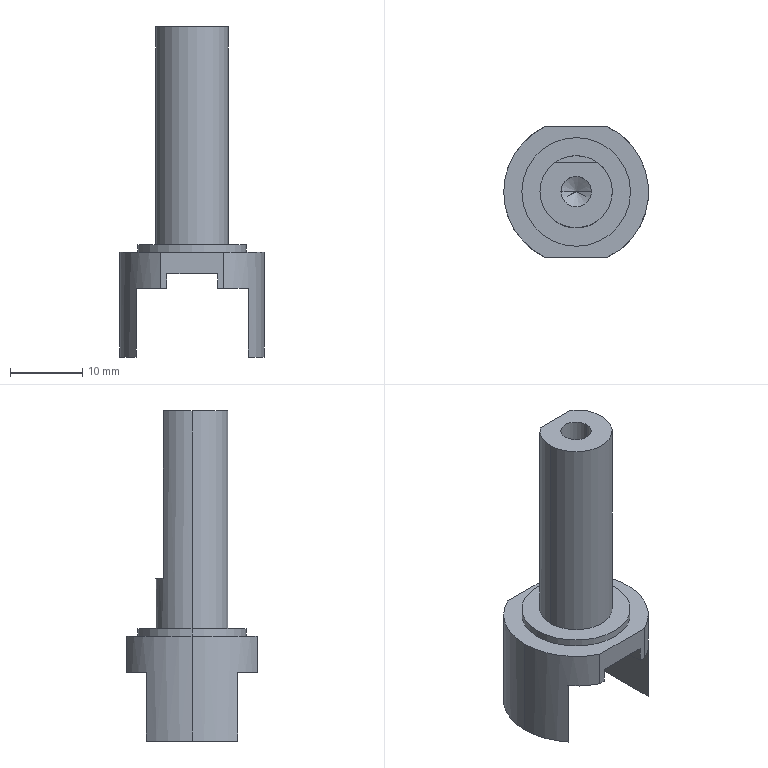Part | STEP file | turning shaft | 1 solid | 27 faces | box 20 x 18 x 45.6 mm | volume 3898 mm3 | plane 16 | cylinder 9 | cone 2 | commonest cylinder face diameters 20 x3 4.2 x2 10 x2 15 x2